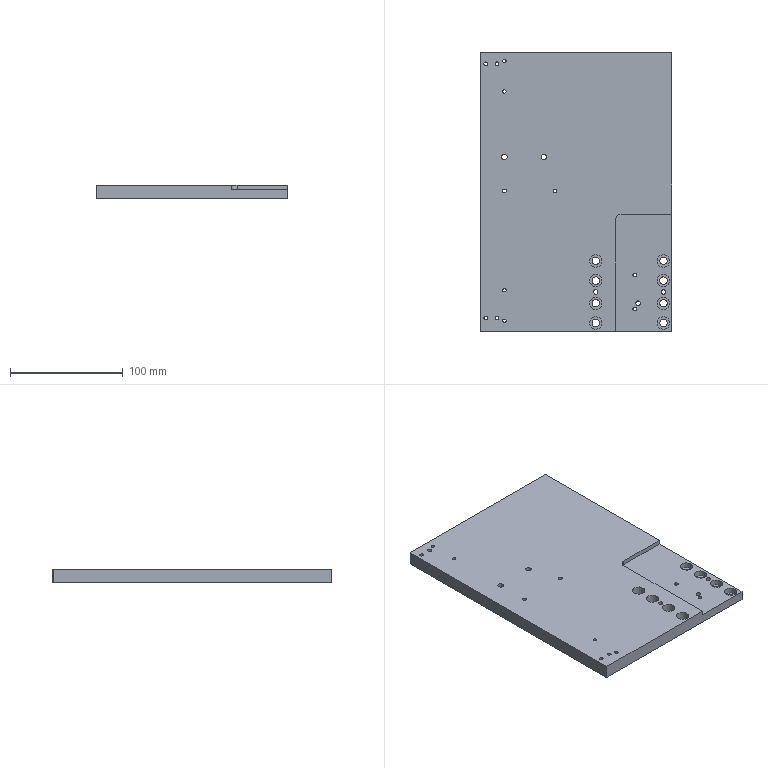Part | 1 solid | 53 faces | box 170 x 247.2 x 12 mm | volume 475967 mm3 | cylinder 34 | plane 19 | commonest cylinder face diameters 3.3 x8 6.6 x8 11 x8 3 x4 4 x3 5 x2
STEP:
#1=CARTESIAN_POINT('',(84.5,-91.3,8.1));
#2=VERTEX_POINT('',#1);
#3=CARTESIAN_POINT('',(85.,-90.8,8.1));
#4=VERTEX_POINT('',#3);
#5=CARTESIAN_POINT('',(85.,-90.8,8.1));
#6=DIRECTION('',(0.7071,0.7071,0.));
#7=VECTOR('',#6,1000.);
#8=LINE('',#5,#7);
#9=EDGE_CURVE('',#2,#4,#8,.T.);
#10=ORIENTED_EDGE('',*,*,#9,.F.);
#11=CARTESIAN_POINT('',(84.5,-91.3,0.));
#12=VERTEX_POINT('',#11);
#13=CARTESIAN_POINT('',(84.5,-91.3,12.));
#14=DIRECTION('',(0.,0.,1.));
#15=VECTOR('',#14,1000.);
#16=LINE('',#13,#15);
#17=EDGE_CURVE('',#12,#2,#16,.T.);
#18=ORIENTED_EDGE('',*,*,#17,.F.);
#19=CARTESIAN_POINT('',(85.,-90.8,0.));
#20=VERTEX_POINT('',#19);
#21=CARTESIAN_POINT('',(87.9,-87.9,0.));
#22=DIRECTION('',(-0.7071,-0.7071,0.));
#23=VECTOR('',#22,1000.);
#24=LINE('',#21,#23);
#25=EDGE_CURVE('',#20,#12,#24,.T.);
#26=ORIENTED_EDGE('',*,*,#25,.F.);
#27=CARTESIAN_POINT('',(85.,-90.8,12.));
#28=DIRECTION('',(0.,0.,-1.));
#29=VECTOR('',#28,1000.);
#30=LINE('',#27,#29);
#31=EDGE_CURVE('',#4,#20,#30,.T.);
#32=ORIENTED_EDGE('',*,*,#31,.F.);
#33=EDGE_LOOP('',(#10,#18,#26,#32));
#34=FACE_BOUND('',#33,.T.);
#35=CARTESIAN_POINT('',(85.,-90.8,12.));
#36=DIRECTION('',(-0.7071,0.7071,0.));
#37=DIRECTION('',(0.,0.,-1.));
#38=AXIS2_PLACEMENT_3D('',#35,#36,#37);
#39=PLANE('',#38);
#40=ADVANCED_FACE('',(#34),#39,.F.);
#41=CARTESIAN_POINT('',(-85.,155.4,0.));
#42=VERTEX_POINT('',#41);
#43=CARTESIAN_POINT('',(-84.5,155.9,0.));
#44=VERTEX_POINT('',#43);
#45=CARTESIAN_POINT('',(-120.2,120.2,0.));
#46=DIRECTION('',(0.7071,0.7071,0.));
#47=VECTOR('',#46,1000.);
#48=LINE('',#45,#47);
#49=EDGE_CURVE('',#42,#44,#48,.T.);
#50=ORIENTED_EDGE('',*,*,#49,.F.);
#51=CARTESIAN_POINT('',(-85.,155.4,12.));
#52=VERTEX_POINT('',#51);
#53=CARTESIAN_POINT('',(-85.,155.4,0.));
#54=DIRECTION('',(0.,0.,-1.));
#55=VECTOR('',#54,1000.);
#56=LINE('',#53,#55);
#57=EDGE_CURVE('',#52,#42,#56,.T.);
#58=ORIENTED_EDGE('',*,*,#57,.F.);
#59=CARTESIAN_POINT('',(-84.5,155.9,12.));
#60=VERTEX_POINT('',#59);
#61=CARTESIAN_POINT('',(-84.5,155.9,12.));
#62=DIRECTION('',(-0.7071,-0.7071,0.));
#63=VECTOR('',#62,1000.);
#64=LINE('',#61,#63);
#65=EDGE_CURVE('',#60,#52,#64,.T.);
#66=ORIENTED_EDGE('',*,*,#65,.F.);
#67=CARTESIAN_POINT('',(-84.5,155.9,12.));
#68=DIRECTION('',(0.,0.,1.));
#69=VECTOR('',#68,1000.);
#70=LINE('',#67,#69);
#71=EDGE_CURVE('',#44,#60,#70,.T.);
#72=ORIENTED_EDGE('',*,*,#71,.F.);
#73=EDGE_LOOP('',(#50,#58,#66,#72));
#74=FACE_BOUND('',#73,.T.);
#75=CARTESIAN_POINT('',(-84.5,155.9,-69.269));
#76=DIRECTION('',(-0.7071,0.7071,0.));
#77=DIRECTION('',(0.,0.,-1.));
#78=AXIS2_PLACEMENT_3D('',#75,#76,#77);
#79=PLANE('',#78);
#80=ADVANCED_FACE('',(#74),#79,.T.);
#81=CARTESIAN_POINT('',(85.,155.9,12.));
#82=VERTEX_POINT('',#81);
#83=CARTESIAN_POINT('',(-85.,155.9,12.));
#84=DIRECTION('',(-1.,0.,0.));
#85=VECTOR('',#84,1000.);
#86=LINE('',#83,#85);
#87=EDGE_CURVE('',#82,#60,#86,.T.);
#88=ORIENTED_EDGE('',*,*,#87,.F.);
#89=CARTESIAN_POINT('',(85.,155.9,0.));
#90=VERTEX_POINT('',#89);
#91=CARTESIAN_POINT('',(85.,155.9,-69.269));
#92=DIRECTION('',(0.,0.,1.));
#93=VECTOR('',#92,1000.);
#94=LINE('',#91,#93);
#95=EDGE_CURVE('',#90,#82,#94,.T.);
#96=ORIENTED_EDGE('',*,*,#95,.F.);
#97=CARTESIAN_POINT('',(-85.,155.9,0.));
#98=DIRECTION('',(-1.,0.,0.));
#99=VECTOR('',#98,1000.);
#100=LINE('',#97,#99);
#101=EDGE_CURVE('',#90,#44,#100,.T.);
#102=ORIENTED_EDGE('',*,*,#101,.T.);
#103=ORIENTED_EDGE('',*,*,#71,.T.);
#104=EDGE_LOOP('',(#88,#96,#102,#103));
#105=FACE_BOUND('',#104,.T.);
#106=CARTESIAN_POINT('',(-85.,155.9,-69.269));
#107=DIRECTION('',(0.,1.,0.));
#108=DIRECTION('',(0.,0.,1.));
#109=AXIS2_PLACEMENT_3D('',#106,#107,#108);
#110=PLANE('',#109);
#111=ADVANCED_FACE('',(#105),#110,.T.);
#112=CARTESIAN_POINT('',(35.1,7.7,8.1));
#113=VERTEX_POINT('',#112);
#114=CARTESIAN_POINT('',(35.1,-91.3,8.1));
#115=VERTEX_POINT('',#114);
#116=CARTESIAN_POINT('',(35.1,0.,8.1));
#117=DIRECTION('',(0.,-1.,0.));
#118=VECTOR('',#117,1000.);
#119=LINE('',#116,#118);
#120=EDGE_CURVE('',#113,#115,#119,.T.);
#121=ORIENTED_EDGE('',*,*,#120,.F.);
#122=CARTESIAN_POINT('',(35.1,7.7,12.));
#123=VERTEX_POINT('',#122);
#124=CARTESIAN_POINT('',(35.1,7.7,8.));
#125=DIRECTION('',(0.,0.,1.));
#126=VECTOR('',#125,1000.);
#127=LINE('',#124,#126);
#128=EDGE_CURVE('',#113,#123,#127,.T.);
#129=ORIENTED_EDGE('',*,*,#128,.T.);
#130=CARTESIAN_POINT('',(35.1,-91.3,12.));
#131=VERTEX_POINT('',#130);
#132=CARTESIAN_POINT('',(35.1,-91.3,12.));
#133=DIRECTION('',(0.,-1.,0.));
#134=VECTOR('',#133,1000.);
#135=LINE('',#132,#134);
#136=EDGE_CURVE('',#123,#131,#135,.T.);
#137=ORIENTED_EDGE('',*,*,#136,.T.);
#138=CARTESIAN_POINT('',(35.1,-91.3,12.));
#139=DIRECTION('',(0.,0.,1.));
#140=VECTOR('',#139,1000.);
#141=LINE('',#138,#140);
#142=EDGE_CURVE('',#115,#131,#141,.T.);
#143=ORIENTED_EDGE('',*,*,#142,.F.);
#144=EDGE_LOOP('',(#121,#129,#137,#143));
#145=FACE_BOUND('',#144,.T.);
#146=CARTESIAN_POINT('',(35.1,-91.3,8.));
#147=DIRECTION('',(-1.,0.,0.));
#148=DIRECTION('',(0.,0.,1.));
#149=AXIS2_PLACEMENT_3D('',#146,#147,#148);
#150=PLANE('',#149);
#151=ADVANCED_FACE('',(#145),#150,.F.);
#152=CARTESIAN_POINT('',(40.1,12.7,8.1));
#153=VERTEX_POINT('',#152);
#154=CARTESIAN_POINT('',(85.,12.7,8.1));
#155=VERTEX_POINT('',#154);
#156=CARTESIAN_POINT('',(0.,12.7,8.1));
#157=DIRECTION('',(1.,0.,0.));
#158=VECTOR('',#157,1000.);
#159=LINE('',#156,#158);
#160=EDGE_CURVE('',#153,#155,#159,.T.);
#161=ORIENTED_EDGE('',*,*,#160,.F.);
#162=CARTESIAN_POINT('',(40.1,7.7,8.1));
#163=DIRECTION('',(0.,0.,1.));
#164=DIRECTION('',(1.,0.,0.));
#165=AXIS2_PLACEMENT_3D('',#162,#163,#164);
#166=CIRCLE('',#165,5.);
#167=EDGE_CURVE('',#153,#113,#166,.T.);
#168=ORIENTED_EDGE('',*,*,#167,.T.);
#169=ORIENTED_EDGE('',*,*,#120,.T.);
#170=CARTESIAN_POINT('',(-85.,-91.3,8.1));
#171=DIRECTION('',(1.,0.,0.));
#172=VECTOR('',#171,1000.);
#173=LINE('',#170,#172);
#174=EDGE_CURVE('',#115,#2,#173,.T.);
#175=ORIENTED_EDGE('',*,*,#174,.T.);
#176=ORIENTED_EDGE('',*,*,#9,.T.);
#177=CARTESIAN_POINT('',(85.,-91.3,8.1));
#178=DIRECTION('',(0.,1.,0.));
#179=VECTOR('',#178,1000.);
#180=LINE('',#177,#179);
#181=EDGE_CURVE('',#4,#155,#180,.T.);
#182=ORIENTED_EDGE('',*,*,#181,.T.);
#183=EDGE_LOOP('',(#161,#168,#169,#175,#176,#182));
#184=FACE_BOUND('',#183,.T.);
#185=CARTESIAN_POINT('',(83.,-28.8,8.1));
#186=VERTEX_POINT('',#185);
#187=CARTESIAN_POINT('',(77.5,-28.8,8.1));
#188=DIRECTION('',(0.,0.,1.));
#189=DIRECTION('',(1.,0.,0.));
#190=AXIS2_PLACEMENT_3D('',#187,#188,#189);
#191=CIRCLE('',#190,5.5);
#192=EDGE_CURVE('',#186,#186,#191,.F.);
#193=ORIENTED_EDGE('',*,*,#192,.T.);
#194=EDGE_LOOP('',(#193));
#195=FACE_BOUND('',#194,.T.);
#196=CARTESIAN_POINT('',(83.,-83.8,8.1));
#197=VERTEX_POINT('',#196);
#198=CARTESIAN_POINT('',(77.5,-83.8,8.1));
#199=DIRECTION('',(0.,0.,1.));
#200=DIRECTION('',(1.,0.,0.));
#201=AXIS2_PLACEMENT_3D('',#198,#199,#200);
#202=CIRCLE('',#201,5.5);
#203=EDGE_CURVE('',#197,#197,#202,.F.);
#204=ORIENTED_EDGE('',*,*,#203,.T.);
#205=EDGE_LOOP('',(#204));
#206=FACE_BOUND('',#205,.T.);
#207=CARTESIAN_POINT('',(83.,-46.3,8.1));
#208=VERTEX_POINT('',#207);
#209=CARTESIAN_POINT('',(77.5,-46.3,8.1));
#210=DIRECTION('',(0.,0.,1.));
#211=DIRECTION('',(1.,0.,0.));
#212=AXIS2_PLACEMENT_3D('',#209,#210,#211);
#213=CIRCLE('',#212,5.5);
#214=EDGE_CURVE('',#208,#208,#213,.F.);
#215=ORIENTED_EDGE('',*,*,#214,.T.);
#216=EDGE_LOOP('',(#215));
#217=FACE_BOUND('',#216,.T.);
#218=CARTESIAN_POINT('',(83.,-66.3,8.1));
#219=VERTEX_POINT('',#218);
#220=CARTESIAN_POINT('',(77.5,-66.3,8.1));
#221=DIRECTION('',(0.,0.,1.));
#222=DIRECTION('',(1.,0.,0.));
#223=AXIS2_PLACEMENT_3D('',#220,#221,#222);
#224=CIRCLE('',#223,5.5);
#225=EDGE_CURVE('',#219,#219,#224,.F.);
#226=ORIENTED_EDGE('',*,*,#225,.T.);
#227=EDGE_LOOP('',(#226));
#228=FACE_BOUND('',#227,.T.);
#229=CARTESIAN_POINT('',(57.,-66.3,8.1));
#230=VERTEX_POINT('',#229);
#231=CARTESIAN_POINT('',(55.,-66.3,8.1));
#232=DIRECTION('',(0.,0.,1.));
#233=DIRECTION('',(1.,0.,0.));
#234=AXIS2_PLACEMENT_3D('',#231,#232,#233);
#235=CIRCLE('',#234,2.);
#236=EDGE_CURVE('',#230,#230,#235,.F.);
#237=ORIENTED_EDGE('',*,*,#236,.T.);
#238=EDGE_LOOP('',(#237));
#239=FACE_BOUND('',#238,.T.);
#240=CARTESIAN_POINT('',(79.5,-56.3,8.1));
#241=VERTEX_POINT('',#240);
#242=CARTESIAN_POINT('',(77.5,-56.3,8.1));
#243=DIRECTION('',(0.,0.,1.));
#244=DIRECTION('',(1.,0.,0.));
#245=AXIS2_PLACEMENT_3D('',#242,#243,#244);
#246=CIRCLE('',#245,2.);
#247=EDGE_CURVE('',#241,#241,#246,.F.);
#248=ORIENTED_EDGE('',*,*,#247,.T.);
#249=EDGE_LOOP('',(#248));
#250=FACE_BOUND('',#249,.T.);
#251=CARTESIAN_POINT('',(53.65,-41.3,8.1));
#252=VERTEX_POINT('',#251);
#253=CARTESIAN_POINT('',(52.,-41.3,8.1));
#254=DIRECTION('',(0.,0.,1.));
#255=DIRECTION('',(1.,0.,0.));
#256=AXIS2_PLACEMENT_3D('',#253,#254,#255);
#257=CIRCLE('',#256,1.65);
#258=EDGE_CURVE('',#252,#252,#257,.T.);
#259=ORIENTED_EDGE('',*,*,#258,.F.);
#260=EDGE_LOOP('',(#259));
#261=FACE_BOUND('',#260,.T.);
#262=CARTESIAN_POINT('',(53.65,-71.3,8.1));
#263=VERTEX_POINT('',#262);
#264=CARTESIAN_POINT('',(52.,-71.3,8.1));
#265=DIRECTION('',(0.,0.,1.));
#266=DIRECTION('',(1.,0.,0.));
#267=AXIS2_PLACEMENT_3D('',#264,#265,#266);
#268=CIRCLE('',#267,1.65);
#269=EDGE_CURVE('',#263,#263,#268,.T.);
#270=ORIENTED_EDGE('',*,*,#269,.F.);
#271=EDGE_LOOP('',(#270));
#272=FACE_BOUND('',#271,.T.);
#273=CARTESIAN_POINT('',(0.,0.,8.1));
#274=DIRECTION('',(0.,0.,1.));
#275=DIRECTION('',(1.,0.,0.));
#276=AXIS2_PLACEMENT_3D('',#273,#274,#275);
#277=PLANE('',#276);
#278=ADVANCED_FACE('',(#184,#195,#206,#217,#228,#239,#250,#261,#272),#277,.T.);
#279=CARTESIAN_POINT('',(83.,-66.3,3.));
#280=VERTEX_POINT('',#279);
#281=CARTESIAN_POINT('',(77.5,-66.3,3.));
#282=DIRECTION('',(0.,0.,1.));
#283=DIRECTION('',(1.,0.,0.));
#284=AXIS2_PLACEMENT_3D('',#281,#282,#283);
#285=CIRCLE('',#284,5.5);
#286=EDGE_CURVE('',#280,#280,#285,.T.);
#287=ORIENTED_EDGE('',*,*,#286,.T.);
#288=EDGE_LOOP('',(#287));
#289=FACE_BOUND('',#288,.T.);
#290=CARTESIAN_POINT('',(80.8,-66.3,3.));
#291=VERTEX_POINT('',#290);
#292=CARTESIAN_POINT('',(77.5,-66.3,3.));
#293=DIRECTION('',(0.,0.,1.));
#294=DIRECTION('',(1.,0.,0.));
#295=AXIS2_PLACEMENT_3D('',#292,#293,#294);
#296=CIRCLE('',#295,3.3);
#297=EDGE_CURVE('',#291,#291,#296,.T.);
#298=ORIENTED_EDGE('',*,*,#297,.F.);
#299=EDGE_LOOP('',(#298));
#300=FACE_BOUND('',#299,.T.);
#301=CARTESIAN_POINT('',(80.8,-66.3,3.));
#302=DIRECTION('',(0.,0.,-1.));
#303=DIRECTION('',(-1.,0.,0.));
#304=AXIS2_PLACEMENT_3D('',#301,#302,#303);
#305=PLANE('',#304);
#306=ADVANCED_FACE('',(#289,#300),#305,.F.);
#307=CARTESIAN_POINT('',(72.,-46.3,3.));
#308=VERTEX_POINT('',#307);
#309=CARTESIAN_POINT('',(77.5,-46.3,3.));
#310=DIRECTION('',(0.,0.,1.));
#311=DIRECTION('',(-1.,0.,0.));
#312=AXIS2_PLACEMENT_3D('',#309,#310,#311);
#313=CIRCLE('',#312,5.5);
#314=EDGE_CURVE('',#308,#308,#313,.T.);
#315=ORIENTED_EDGE('',*,*,#314,.T.);
#316=EDGE_LOOP('',(#315));
#317=FACE_BOUND('',#316,.T.);
#318=CARTESIAN_POINT('',(74.2,-46.3,3.));
#319=VERTEX_POINT('',#318);
#320=CARTESIAN_POINT('',(77.5,-46.3,3.));
#321=DIRECTION('',(0.,0.,1.));
#322=DIRECTION('',(-1.,0.,0.));
#323=AXIS2_PLACEMENT_3D('',#320,#321,#322);
#324=CIRCLE('',#323,3.3);
#325=EDGE_CURVE('',#319,#319,#324,.T.);
#326=ORIENTED_EDGE('',*,*,#325,.F.);
#327=EDGE_LOOP('',(#326));
#328=FACE_BOUND('',#327,.T.);
#329=CARTESIAN_POINT('',(80.8,-66.3,3.));
#330=DIRECTION('',(0.,0.,-1.));
#331=DIRECTION('',(-1.,0.,0.));
#332=AXIS2_PLACEMENT_3D('',#329,#330,#331);
#333=PLANE('',#332);
#334=ADVANCED_FACE('',(#317,#328),#333,.F.);
#335=CARTESIAN_POINT('',(12.,-66.3,3.));
#336=VERTEX_POINT('',#335);
#337=CARTESIAN_POINT('',(17.5,-66.3,3.));
#338=DIRECTION('',(0.,0.,1.));
#339=DIRECTION('',(-1.,0.,0.));
#340=AXIS2_PLACEMENT_3D('',#337,#338,#339);
#341=CIRCLE('',#340,5.5);
#342=EDGE_CURVE('',#336,#336,#341,.T.);
#343=ORIENTED_EDGE('',*,*,#342,.T.);
#344=EDGE_LOOP('',(#343));
#345=FACE_BOUND('',#344,.T.);
#346=CARTESIAN_POINT('',(14.2,-66.3,3.));
#347=VERTEX_POINT('',#346);
#348=CARTESIAN_POINT('',(17.5,-66.3,3.));
#349=DIRECTION('',(0.,0.,1.));
#350=DIRECTION('',(-1.,0.,0.));
#351=AXIS2_PLACEMENT_3D('',#348,#349,#350);
#352=CIRCLE('',#351,3.3);
#353=EDGE_CURVE('',#347,#347,#352,.T.);
#354=ORIENTED_EDGE('',*,*,#353,.F.);
#355=EDGE_LOOP('',(#354));
#356=FACE_BOUND('',#355,.T.);
#357=CARTESIAN_POINT('',(80.8,-66.3,3.));
#358=DIRECTION('',(0.,0.,-1.));
#359=DIRECTION('',(-1.,0.,0.));
#360=AXIS2_PLACEMENT_3D('',#357,#358,#359);
#361=PLANE('',#360);
#362=ADVANCED_FACE('',(#345,#356),#361,.F.);
#363=CARTESIAN_POINT('',(12.,-46.3,3.));
#364=VERTEX_POINT('',#363);
#365=CARTESIAN_POINT('',(17.5,-46.3,3.));
#366=DIRECTION('',(0.,0.,1.));
#367=DIRECTION('',(-1.,0.,0.));
#368=AXIS2_PLACEMENT_3D('',#365,#366,#367);
#369=CIRCLE('',#368,5.5);
#370=EDGE_CURVE('',#364,#364,#369,.T.);
#371=ORIENTED_EDGE('',*,*,#370,.T.);
#372=EDGE_LOOP('',(#371));
#373=FACE_BOUND('',#372,.T.);
#374=CARTESIAN_POINT('',(14.2,-46.3,3.));
#375=VERTEX_POINT('',#374);
#376=CARTESIAN_POINT('',(17.5,-46.3,3.));
#377=DIRECTION('',(0.,0.,1.));
#378=DIRECTION('',(-1.,0.,0.));
#379=AXIS2_PLACEMENT_3D('',#376,#377,#378);
#380=CIRCLE('',#379,3.3);
#381=EDGE_CURVE('',#375,#375,#380,.T.);
#382=ORIENTED_EDGE('',*,*,#381,.F.);
#383=EDGE_LOOP('',(#382));
#384=FACE_BOUND('',#383,.T.);
#385=CARTESIAN_POINT('',(80.8,-66.3,3.));
#386=DIRECTION('',(0.,0.,-1.));
#387=DIRECTION('',(-1.,0.,0.));
#388=AXIS2_PLACEMENT_3D('',#385,#386,#387);
#389=PLANE('',#388);
#390=ADVANCED_FACE('',(#373,#384),#389,.F.);
#391=CARTESIAN_POINT('',(72.,-83.8,3.));
#392=VERTEX_POINT('',#391);
#393=CARTESIAN_POINT('',(77.5,-83.8,3.));
#394=DIRECTION('',(0.,0.,1.));
#395=DIRECTION('',(-1.,0.,0.));
#396=AXIS2_PLACEMENT_3D('',#393,#394,#395);
#397=CIRCLE('',#396,5.5);
#398=EDGE_CURVE('',#392,#392,#397,.T.);
#399=ORIENTED_EDGE('',*,*,#398,.T.);
#400=EDGE_LOOP('',(#399));
#401=FACE_BOUND('',#400,.T.);
#402=CARTESIAN_POINT('',(74.2,-83.8,3.));
#403=VERTEX_POINT('',#402);
#404=CARTESIAN_POINT('',(77.5,-83.8,3.));
#405=DIRECTION('',(0.,0.,1.));
#406=DIRECTION('',(-1.,0.,0.));
#407=AXIS2_PLACEMENT_3D('',#404,#405,#406);
#408=CIRCLE('',#407,3.3);
#409=EDGE_CURVE('',#403,#403,#408,.T.);
#410=ORIENTED_EDGE('',*,*,#409,.F.);
#411=EDGE_LOOP('',(#410));
#412=FACE_BOUND('',#411,.T.);
#413=CARTESIAN_POINT('',(80.8,-66.3,3.));
#414=DIRECTION('',(0.,0.,-1.));
#415=DIRECTION('',(-1.,0.,0.));
#416=AXIS2_PLACEMENT_3D('',#413,#414,#415);
#417=PLANE('',#416);
#418=ADVANCED_FACE('',(#401,#412),#417,.F.);
#419=CARTESIAN_POINT('',(12.,-83.8,3.));
#420=VERTEX_POINT('',#419);
#421=CARTESIAN_POINT('',(17.5,-83.8,3.));
#422=DIRECTION('',(0.,0.,1.));
#423=DIRECTION('',(-1.,0.,0.));
#424=AXIS2_PLACEMENT_3D('',#421,#422,#423);
#425=CIRCLE('',#424,5.5);
#426=EDGE_CURVE('',#420,#420,#425,.T.);
#427=ORIENTED_EDGE('',*,*,#426,.T.);
#428=EDGE_LOOP('',(#427));
#429=FACE_BOUND('',#428,.T.);
#430=CARTESIAN_POINT('',(14.2,-83.8,3.));
#431=VERTEX_POINT('',#430);
#432=CARTESIAN_POINT('',(17.5,-83.8,3.));
#433=DIRECTION('',(0.,0.,1.));
#434=DIRECTION('',(-1.,0.,0.));
#435=AXIS2_PLACEMENT_3D('',#432,#433,#434);
#436=CIRCLE('',#435,3.3);
#437=EDGE_CURVE('',#431,#431,#436,.T.);
#438=ORIENTED_EDGE('',*,*,#437,.F.);
#439=EDGE_LOOP('',(#438));
#440=FACE_BOUND('',#439,.T.);
#441=CARTESIAN_POINT('',(80.8,-66.3,3.));
#442=DIRECTION('',(0.,0.,-1.));
#443=DIRECTION('',(-1.,0.,0.));
#444=AXIS2_PLACEMENT_3D('',#441,#442,#443);
#445=PLANE('',#444);
#446=ADVANCED_FACE('',(#429,#440),#445,.F.);
#447=CARTESIAN_POINT('',(72.,-28.8,3.));
#448=VERTEX_POINT('',#447);
#449=CARTESIAN_POINT('',(77.5,-28.8,3.));
#450=DIRECTION('',(0.,0.,1.));
#451=DIRECTION('',(-1.,0.,0.));
#452=AXIS2_PLACEMENT_3D('',#449,#450,#451);
#453=CIRCLE('',#452,5.5);
#454=EDGE_CURVE('',#448,#448,#453,.T.);
#455=ORIENTED_EDGE('',*,*,#454,.T.);
#456=EDGE_LOOP('',(#455));
#457=FACE_BOUND('',#456,.T.);
#458=CARTESIAN_POINT('',(74.2,-28.8,3.));
#459=VERTEX_POINT('',#458);
#460=CARTESIAN_POINT('',(77.5,-28.8,3.));
#461=DIRECTION('',(0.,0.,1.));
#462=DIRECTION('',(-1.,0.,0.));
#463=AXIS2_PLACEMENT_3D('',#460,#461,#462);
#464=CIRCLE('',#463,3.3);
#465=EDGE_CURVE('',#459,#459,#464,.T.);
#466=ORIENTED_EDGE('',*,*,#465,.F.);
#467=EDGE_LOOP('',(#466));
#468=FACE_BOUND('',#467,.T.);
#469=CARTESIAN_POINT('',(80.8,-66.3,3.));
#470=DIRECTION('',(0.,0.,-1.));
#471=DIRECTION('',(-1.,0.,0.));
#472=AXIS2_PLACEMENT_3D('',#469,#470,#471);
#473=PLANE('',#472);
#474=ADVANCED_FACE('',(#457,#468),#473,.F.);
#475=CARTESIAN_POINT('',(12.,-28.8,3.));
#476=VERTEX_POINT('',#475);
#477=CARTESIAN_POINT('',(17.5,-28.8,3.));
#478=DIRECTION('',(0.,0.,1.));
#479=DIRECTION('',(-1.,0.,0.));
#480=AXIS2_PLACEMENT_3D('',#477,#478,#479);
#481=CIRCLE('',#480,5.5);
#482=EDGE_CURVE('',#476,#476,#481,.T.);
#483=ORIENTED_EDGE('',*,*,#482,.T.);
#484=EDGE_LOOP('',(#483));
#485=FACE_BOUND('',#484,.T.);
#486=CARTESIAN_POINT('',(14.2,-28.8,3.));
#487=VERTEX_POINT('',#486);
#488=CARTESIAN_POINT('',(17.5,-28.8,3.));
#489=DIRECTION('',(0.,0.,1.));
#490=DIRECTION('',(-1.,0.,0.));
#491=AXIS2_PLACEMENT_3D('',#488,#489,#490);
#492=CIRCLE('',#491,3.3);
#493=EDGE_CURVE('',#487,#487,#492,.T.);
#494=ORIENTED_EDGE('',*,*,#493,.F.);
#495=EDGE_LOOP('',(#494));
#496=FACE_BOUND('',#495,.T.);
#497=CARTESIAN_POINT('',(80.8,-66.3,3.));
#498=DIRECTION('',(0.,0.,-1.));
#499=DIRECTION('',(-1.,0.,0.));
#500=AXIS2_PLACEMENT_3D('',#497,#498,#499);
#501=PLANE('',#500);
#502=ADVANCED_FACE('',(#485,#496),#501,.F.);
#503=CARTESIAN_POINT('',(-85.,-91.3,0.));
#504=VERTEX_POINT('',#503);
#505=CARTESIAN_POINT('',(-85.,-91.3,0.));
#506=DIRECTION('',(1.,0.,0.));
#507=VECTOR('',#506,1000.);
#508=LINE('',#505,#507);
#509=EDGE_CURVE('',#504,#12,#508,.T.);
#510=ORIENTED_EDGE('',*,*,#509,.T.);
#511=ORIENTED_EDGE('',*,*,#17,.T.);
#512=ORIENTED_EDGE('',*,*,#174,.F.);
#513=ORIENTED_EDGE('',*,*,#142,.T.);
#514=CARTESIAN_POINT('',(-85.,-91.3,12.));
#515=VERTEX_POINT('',#514);
#516=CARTESIAN_POINT('',(-85.,-91.3,12.));
#517=DIRECTION('',(1.,0.,0.));
#518=VECTOR('',#517,1000.);
#519=LINE('',#516,#518);
#520=EDGE_CURVE('',#515,#131,#519,.T.);
#521=ORIENTED_EDGE('',*,*,#520,.F.);
#522=CARTESIAN_POINT('',(-85.,-91.3,12.));
#523=DIRECTION('',(0.,0.,-1.));
#524=VECTOR('',#523,1000.);
#525=LINE('',#522,#524);
#526=EDGE_CURVE('',#515,#504,#525,.T.);
#527=ORIENTED_EDGE('',*,*,#526,.T.);
#528=EDGE_LOOP('',(#510,#511,#512,#513,#521,#527));
#529=FACE_BOUND('',#528,.T.);
#530=CARTESIAN_POINT('',(-85.,-91.3,12.));
#531=DIRECTION('',(0.,1.,0.));
#532=DIRECTION('',(0.,0.,1.));
#533=AXIS2_PLACEMENT_3D('',#530,#531,#532);
#534=PLANE('',#533);
#535=ADVANCED_FACE('',(#529),#534,.F.);
#536=CARTESIAN_POINT('',(-85.,-91.3,12.));
#537=DIRECTION('',(0.,-1.,0.));
#538=VECTOR('',#537,1000.);
#539=LINE('',#536,#538);
#540=EDGE_CURVE('',#52,#515,#539,.T.);
#541=ORIENTED_EDGE('',*,*,#540,.F.);
#542=ORIENTED_EDGE('',*,*,#57,.T.);
#543=CARTESIAN_POINT('',(-85.,-91.3,0.));
#544=DIRECTION('',(0.,-1.,0.));
#545=VECTOR('',#544,1000.);
#546=LINE('',#543,#545);
#547=EDGE_CURVE('',#42,#504,#546,.T.);
#548=ORIENTED_EDGE('',*,*,#547,.T.);
#549=ORIENTED_EDGE('',*,*,#526,.F.);
#550=EDGE_LOOP('',(#541,#542,#548,#549));
#551=FACE_BOUND('',#550,.T.);
#552=CARTESIAN_POINT('',(-85.,-91.3,12.));
#553=DIRECTION('',(1.,0.,0.));
#554=DIRECTION('',(0.,0.,-1.));
#555=AXIS2_PLACEMENT_3D('',#552,#553,#554);
#556=PLANE('',#555);
#557=ADVANCED_FACE('',(#551),#556,.F.);
#558=CARTESIAN_POINT('',(85.,-91.3,0.));
#559=DIRECTION('',(0.,1.,0.));
#560=VECTOR('',#559,1000.);
#561=LINE('',#558,#560);
#562=EDGE_CURVE('',#20,#90,#561,.T.);
#563=ORIENTED_EDGE('',*,*,#562,.T.);
#564=ORIENTED_EDGE('',*,*,#95,.T.);
#565=CARTESIAN_POINT('',(85.,12.7,12.));
#566=VERTEX_POINT('',#565);
#567=CARTESIAN_POINT('',(85.,32.3,12.));
#568=DIRECTION('',(0.,-1.,0.));
#569=VECTOR('',#568,1000.);
#570=LINE('',#567,#569);
#571=EDGE_CURVE('',#82,#566,#570,.T.);
#572=ORIENTED_EDGE('',*,*,#571,.T.);
#573=CARTESIAN_POINT('',(85.,12.7,8.));
#574=DIRECTION('',(0.,0.,1.));
#575=VECTOR('',#574,1000.);
#576=LINE('',#573,#575);
#577=EDGE_CURVE('',#155,#566,#576,.T.);
#578=ORIENTED_EDGE('',*,*,#577,.F.);
#579=ORIENTED_EDGE('',*,*,#181,.F.);
#580=ORIENTED_EDGE('',*,*,#31,.T.);
#581=EDGE_LOOP('',(#563,#564,#572,#578,#579,#580));
#582=FACE_BOUND('',#581,.T.);
#583=CARTESIAN_POINT('',(85.,-91.3,12.));
#584=DIRECTION('',(-1.,0.,0.));
#585=DIRECTION('',(0.,0.,1.));
#586=AXIS2_PLACEMENT_3D('',#583,#584,#585);
#587=PLANE('',#586);
#588=ADVANCED_FACE('',(#582),#587,.F.);
#589=ORIENTED_EDGE('',*,*,#136,.F.);
#590=CARTESIAN_POINT('',(40.1,12.7,12.));
#591=VERTEX_POINT('',#590);
#592=CARTESIAN_POINT('',(40.1,7.7,12.));
#593=DIRECTION('',(0.,0.,-1.));
#594=DIRECTION('',(-1.,0.,0.));
#595=AXIS2_PLACEMENT_3D('',#592,#593,#594);
#596=CIRCLE('',#595,5.);
#597=EDGE_CURVE('',#123,#591,#596,.T.);
#598=ORIENTED_EDGE('',*,*,#597,.T.);
#599=CARTESIAN_POINT('',(60.,12.7,12.));
#600=DIRECTION('',(-1.,0.,0.));
#601=VECTOR('',#600,1000.);
#602=LINE('',#599,#601);
#603=EDGE_CURVE('',#566,#591,#602,.T.);
#604=ORIENTED_EDGE('',*,*,#603,.F.);
#605=ORIENTED_EDGE('',*,*,#571,.F.);
#606=ORIENTED_EDGE('',*,*,#87,.T.);
#607=ORIENTED_EDGE('',*,*,#65,.T.);
#608=ORIENTED_EDGE('',*,*,#540,.T.);
#609=ORIENTED_EDGE('',*,*,#520,.T.);
#610=EDGE_LOOP('',(#589,#598,#604,#605,#606,#607,#608,#609));
#611=FACE_BOUND('',#610,.T.);
#612=CARTESIAN_POINT('',(-68.35,145.9,12.));
#613=VERTEX_POINT('',#612);
#614=CARTESIAN_POINT('',(-70.,145.9,12.));
#615=DIRECTION('',(0.,0.,1.));
#616=DIRECTION('',(1.,0.,0.));
#617=AXIS2_PLACEMENT_3D('',#614,#615,#616);
#618=CIRCLE('',#617,1.65);
#619=EDGE_CURVE('',#613,#613,#618,.T.);
#620=ORIENTED_EDGE('',*,*,#619,.F.);
#621=EDGE_LOOP('',(#620));
#622=FACE_BOUND('',#621,.T.);
#623=CARTESIAN_POINT('',(-61.,63.3,12.));
#624=VERTEX_POINT('',#623);
#625=CARTESIAN_POINT('',(-63.5,63.3,12.));
#626=DIRECTION('',(0.,0.,1.));
#627=DIRECTION('',(1.,0.,0.));
#628=AXIS2_PLACEMENT_3D('',#625,#626,#627);
#629=CIRCLE('',#628,2.5);
#630=EDGE_CURVE('',#624,#624,#629,.T.);
#631=ORIENTED_EDGE('',*,*,#630,.F.);
#632=EDGE_LOOP('',(#631));
#633=FACE_BOUND('',#632,.T.);
#634=CARTESIAN_POINT('',(23.,-28.8,12.));
#635=VERTEX_POINT('',#634);
#636=CARTESIAN_POINT('',(17.5,-28.8,12.));
#637=DIRECTION('',(0.,0.,1.));
#638=DIRECTION('',(1.,0.,0.));
#639=AXIS2_PLACEMENT_3D('',#636,#637,#638);
#640=CIRCLE('',#639,5.5);
#641=EDGE_CURVE('',#635,#635,#640,.T.);
#642=ORIENTED_EDGE('',*,*,#641,.F.);
#643=EDGE_LOOP('',(#642));
#644=FACE_BOUND('',#643,.T.);
#645=CARTESIAN_POINT('',(23.,-83.8,12.));
#646=VERTEX_POINT('',#645);
#647=CARTESIAN_POINT('',(17.5,-83.8,12.));
#648=DIRECTION('',(0.,0.,1.));
#649=DIRECTION('',(1.,0.,0.));
#650=AXIS2_PLACEMENT_3D('',#647,#648,#649);
#651=CIRCLE('',#650,5.5);
#652=EDGE_CURVE('',#646,#646,#651,.T.);
#653=ORIENTED_EDGE('',*,*,#652,.F.);
#654=EDGE_LOOP('',(#653));
#655=FACE_BOUND('',#654,.T.);
#656=CARTESIAN_POINT('',(23.,-46.3,12.));
#657=VERTEX_POINT('',#656);
#658=CARTESIAN_POINT('',(17.5,-46.3,12.));
#659=DIRECTION('',(0.,0.,1.));
#660=DIRECTION('',(1.,0.,0.));
#661=AXIS2_PLACEMENT_3D('',#658,#659,#660);
#662=CIRCLE('',#661,5.5);
#663=EDGE_CURVE('',#657,#657,#662,.T.);
#664=ORIENTED_EDGE('',*,*,#663,.F.);
#665=EDGE_LOOP('',(#664));
#666=FACE_BOUND('',#665,.T.);
#667=CARTESIAN_POINT('',(23.,-66.3,12.));
#668=VERTEX_POINT('',#667);
#669=CARTESIAN_POINT('',(17.5,-66.3,12.));
#670=DIRECTION('',(0.,0.,1.));
#671=DIRECTION('',(1.,0.,0.));
#672=AXIS2_PLACEMENT_3D('',#669,#670,#671);
#673=CIRCLE('',#672,5.5);
#674=EDGE_CURVE('',#668,#668,#673,.T.);
#675=ORIENTED_EDGE('',*,*,#674,.F.);
#676=EDGE_LOOP('',(#675));
#677=FACE_BOUND('',#676,.T.);
#678=CARTESIAN_POINT('',(19.5,-56.3,12.));
#679=VERTEX_POINT('',#678);
#680=CARTESIAN_POINT('',(17.5,-56.3,12.));
#681=DIRECTION('',(0.,0.,1.));
#682=DIRECTION('',(1.,0.,0.));
#683=AXIS2_PLACEMENT_3D('',#680,#681,#682);
#684=CIRCLE('',#683,2.);
#685=EDGE_CURVE('',#679,#679,#684,.T.);
#686=ORIENTED_EDGE('',*,*,#685,.F.);
#687=EDGE_LOOP('',(#686));
#688=FACE_BOUND('',#687,.T.);
#689=CARTESIAN_POINT('',(-16.85,33.3,12.));
#690=VERTEX_POINT('',#689);
#691=CARTESIAN_POINT('',(-18.5,33.3,12.));
#692=DIRECTION('',(0.,0.,1.));
#693=DIRECTION('',(1.,0.,0.));
#694=AXIS2_PLACEMENT_3D('',#691,#692,#693);
#695=CIRCLE('',#694,1.65);
#696=EDGE_CURVE('',#690,#690,#695,.T.);
#697=ORIENTED_EDGE('',*,*,#696,.F.);
#698=EDGE_LOOP('',(#697));
#699=FACE_BOUND('',#698,.T.);
#700=CARTESIAN_POINT('',(-61.85,33.3,12.));
#701=VERTEX_POINT('',#700);
#702=CARTESIAN_POINT('',(-63.5,33.3,12.));
#703=DIRECTION('',(0.,0.,1.));
#704=DIRECTION('',(1.,0.,0.));
#705=AXIS2_PLACEMENT_3D('',#702,#703,#704);
#706=CIRCLE('',#705,1.65);
#707=EDGE_CURVE('',#701,#701,#706,.T.);
#708=ORIENTED_EDGE('',*,*,#707,.F.);
#709=EDGE_LOOP('',(#708));
#710=FACE_BOUND('',#709,.T.);
#711=CARTESIAN_POINT('',(-26.,63.3,12.));
#712=VERTEX_POINT('',#711);
#713=CARTESIAN_POINT('',(-28.5,63.3,12.));
#714=DIRECTION('',(0.,0.,1.));
#715=DIRECTION('',(1.,0.,0.));
#716=AXIS2_PLACEMENT_3D('',#713,#714,#715);
#717=CIRCLE('',#716,2.5);
#718=EDGE_CURVE('',#712,#712,#717,.T.);
#719=ORIENTED_EDGE('',*,*,#718,.F.);
#720=EDGE_LOOP('',(#719));
#721=FACE_BOUND('',#720,.T.);
#722=CARTESIAN_POINT('',(-78.35,145.9,12.));
#723=VERTEX_POINT('',#722);
#724=CARTESIAN_POINT('',(-80.,145.9,12.));
#725=DIRECTION('',(0.,0.,1.));
#726=DIRECTION('',(1.,0.,0.));
#727=AXIS2_PLACEMENT_3D('',#724,#725,#726);
#728=CIRCLE('',#727,1.65);
#729=EDGE_CURVE('',#723,#723,#728,.T.);
#730=ORIENTED_EDGE('',*,*,#729,.F.);
#731=EDGE_LOOP('',(#730));
#732=FACE_BOUND('',#731,.T.);
#733=CARTESIAN_POINT('',(-68.35,-79.3,12.));
#734=VERTEX_POINT('',#733);
#735=CARTESIAN_POINT('',(-70.,-79.3,12.));
#736=DIRECTION('',(0.,0.,1.));
#737=DIRECTION('',(1.,0.,0.));
#738=AXIS2_PLACEMENT_3D('',#735,#736,#737);
#739=CIRCLE('',#738,1.65);
#740=EDGE_CURVE('',#734,#734,#739,.T.);
#741=ORIENTED_EDGE('',*,*,#740,.F.);
#742=EDGE_LOOP('',(#741));
#743=FACE_BOUND('',#742,.T.);
#744=CARTESIAN_POINT('',(-78.35,-79.3,12.));
#745=VERTEX_POINT('',#744);
#746=CARTESIAN_POINT('',(-80.,-79.3,12.));
#747=DIRECTION('',(0.,0.,1.));
#748=DIRECTION('',(1.,0.,0.));
#749=AXIS2_PLACEMENT_3D('',#746,#747,#748);
#750=CIRCLE('',#749,1.65);
#751=EDGE_CURVE('',#745,#745,#750,.T.);
#752=ORIENTED_EDGE('',*,*,#751,.F.);
#753=EDGE_LOOP('',(#752));
#754=FACE_BOUND('',#753,.T.);
#755=CARTESIAN_POINT('',(-62.,121.4,12.));
#756=VERTEX_POINT('',#755);
#757=CARTESIAN_POINT('',(-63.5,121.4,12.));
#758=DIRECTION('',(0.,0.,1.));
#759=DIRECTION('',(1.,0.,0.));
#760=AXIS2_PLACEMENT_3D('',#757,#758,#759);
#761=CIRCLE('',#760,1.5);
#762=EDGE_CURVE('',#756,#756,#761,.T.);
#763=ORIENTED_EDGE('',*,*,#762,.F.);
#764=EDGE_LOOP('',(#763));
#765=FACE_BOUND('',#764,.T.);
#766=CARTESIAN_POINT('',(-62.,148.4,12.));
#767=VERTEX_POINT('',#766);
#768=CARTESIAN_POINT('',(-63.5,148.4,12.));
#769=DIRECTION('',(0.,0.,1.));
#770=DIRECTION('',(1.,0.,0.));
#771=AXIS2_PLACEMENT_3D('',#768,#769,#770);
#772=CIRCLE('',#771,1.5);
#773=EDGE_CURVE('',#767,#767,#772,.T.);
#774=ORIENTED_EDGE('',*,*,#773,.F.);
#775=EDGE_LOOP('',(#774));
#776=FACE_BOUND('',#775,.T.);
#777=CARTESIAN_POINT('',(-62.,-54.8,12.));
#778=VERTEX_POINT('',#777);
#779=CARTESIAN_POINT('',(-63.5,-54.8,12.));
#780=DIRECTION('',(0.,0.,1.));
#781=DIRECTION('',(1.,0.,0.));
#782=AXIS2_PLACEMENT_3D('',#779,#780,#781);
#783=CIRCLE('',#782,1.5);
#784=EDGE_CURVE('',#778,#778,#783,.T.);
#785=ORIENTED_EDGE('',*,*,#784,.F.);
#786=EDGE_LOOP('',(#785));
#787=FACE_BOUND('',#786,.T.);
#788=CARTESIAN_POINT('',(-62.,-81.8,12.));
#789=VERTEX_POINT('',#788);
#790=CARTESIAN_POINT('',(-63.5,-81.8,12.));
#791=DIRECTION('',(0.,0.,1.));
#792=DIRECTION('',(1.,0.,0.));
#793=AXIS2_PLACEMENT_3D('',#790,#791,#792);
#794=CIRCLE('',#793,1.5);
#795=EDGE_CURVE('',#789,#789,#794,.T.);
#796=ORIENTED_EDGE('',*,*,#795,.F.);
#797=EDGE_LOOP('',(#796));
#798=FACE_BOUND('',#797,.T.);
#799=CARTESIAN_POINT('',(0.,0.,12.));
#800=DIRECTION('',(0.,0.,-1.));
#801=DIRECTION('',(-1.,0.,0.));
#802=AXIS2_PLACEMENT_3D('',#799,#800,#801);
#803=PLANE('',#802);
#804=ADVANCED_FACE('',(#611,#622,#633,#644,#655,#666,#677,#688,#699,#710,#721,#732,#743,#754,#765,#776,#787,#798),#803,.F.);
#805=CARTESIAN_POINT('',(-78.35,-79.3,0.));
#806=VERTEX_POINT('',#805);
#807=CARTESIAN_POINT('',(-80.,-79.3,0.));
#808=DIRECTION('',(0.,0.,1.));
#809=DIRECTION('',(1.,0.,0.));
#810=AXIS2_PLACEMENT_3D('',#807,#808,#809);
#811=CIRCLE('',#810,1.65);
#812=EDGE_CURVE('',#806,#806,#811,.T.);
#813=ORIENTED_EDGE('',*,*,#812,.T.);
#814=EDGE_LOOP('',(#813));
#815=FACE_BOUND('',#814,.T.);
#816=CARTESIAN_POINT('',(-68.35,-79.3,0.));
#817=VERTEX_POINT('',#816);
#818=CARTESIAN_POINT('',(-70.,-79.3,0.));
#819=DIRECTION('',(0.,0.,1.));
#820=DIRECTION('',(1.,0.,0.));
#821=AXIS2_PLACEMENT_3D('',#818,#819,#820);
#822=CIRCLE('',#821,1.65);
#823=EDGE_CURVE('',#817,#817,#822,.T.);
#824=ORIENTED_EDGE('',*,*,#823,.T.);
#825=EDGE_LOOP('',(#824));
#826=FACE_BOUND('',#825,.T.);
#827=CARTESIAN_POINT('',(-68.35,145.9,0.));
#828=VERTEX_POINT('',#827);
#829=CARTESIAN_POINT('',(-70.,145.9,0.));
#830=DIRECTION('',(0.,0.,1.));
#831=DIRECTION('',(1.,0.,0.));
#832=AXIS2_PLACEMENT_3D('',#829,#830,#831);
#833=CIRCLE('',#832,1.65);
#834=EDGE_CURVE('',#828,#828,#833,.T.);
#835=ORIENTED_EDGE('',*,*,#834,.T.);
#836=EDGE_LOOP('',(#835));
#837=FACE_BOUND('',#836,.T.);
#838=CARTESIAN_POINT('',(80.8,-46.3,0.));
#839=VERTEX_POINT('',#838);
#840=CARTESIAN_POINT('',(77.5,-46.3,0.));
#841=DIRECTION('',(0.,0.,1.));
#842=DIRECTION('',(1.,0.,0.));
#843=AXIS2_PLACEMENT_3D('',#840,#841,#842);
#844=CIRCLE('',#843,3.3);
#845=EDGE_CURVE('',#839,#839,#844,.T.);
#846=ORIENTED_EDGE('',*,*,#845,.T.);
#847=EDGE_LOOP('',(#846));
#848=FACE_BOUND('',#847,.T.);
#849=CARTESIAN_POINT('',(20.8,-66.3,0.));
#850=VERTEX_POINT('',#849);
#851=CARTESIAN_POINT('',(17.5,-66.3,0.));
#852=DIRECTION('',(0.,0.,1.));
#853=DIRECTION('',(1.,0.,0.));
#854=AXIS2_PLACEMENT_3D('',#851,#852,#853);
#855=CIRCLE('',#854,3.3);
#856=EDGE_CURVE('',#850,#850,#855,.T.);
#857=ORIENTED_EDGE('',*,*,#856,.T.);
#858=EDGE_LOOP('',(#857));
#859=FACE_BOUND('',#858,.T.);
#860=CARTESIAN_POINT('',(20.8,-46.3,0.));
#861=VERTEX_POINT('',#860);
#862=CARTESIAN_POINT('',(17.5,-46.3,0.));
#863=DIRECTION('',(0.,0.,1.));
#864=DIRECTION('',(1.,0.,0.));
#865=AXIS2_PLACEMENT_3D('',#862,#863,#864);
#866=CIRCLE('',#865,3.3);
#867=EDGE_CURVE('',#861,#861,#866,.T.);
#868=ORIENTED_EDGE('',*,*,#867,.T.);
#869=EDGE_LOOP('',(#868));
#870=FACE_BOUND('',#869,.T.);
#871=CARTESIAN_POINT('',(80.8,-83.8,0.));
#872=VERTEX_POINT('',#871);
#873=CARTESIAN_POINT('',(77.5,-83.8,0.));
#874=DIRECTION('',(0.,0.,1.));
#875=DIRECTION('',(1.,0.,0.));
#876=AXIS2_PLACEMENT_3D('',#873,#874,#875);
#877=CIRCLE('',#876,3.3);
#878=EDGE_CURVE('',#872,#872,#877,.T.);
#879=ORIENTED_EDGE('',*,*,#878,.T.);
#880=EDGE_LOOP('',(#879));
#881=FACE_BOUND('',#880,.T.);
#882=CARTESIAN_POINT('',(20.8,-83.8,0.));
#883=VERTEX_POINT('',#882);
#884=CARTESIAN_POINT('',(17.5,-83.8,0.));
#885=DIRECTION('',(0.,0.,1.));
#886=DIRECTION('',(1.,0.,0.));
#887=AXIS2_PLACEMENT_3D('',#884,#885,#886);
#888=CIRCLE('',#887,3.3);
#889=EDGE_CURVE('',#883,#883,#888,.T.);
#890=ORIENTED_EDGE('',*,*,#889,.T.);
#891=EDGE_LOOP('',(#890));
#892=FACE_BOUND('',#891,.T.);
#893=CARTESIAN_POINT('',(80.8,-28.8,0.));
#894=VERTEX_POINT('',#893);
#895=CARTESIAN_POINT('',(77.5,-28.8,0.));
#896=DIRECTION('',(0.,0.,1.));
#897=DIRECTION('',(1.,0.,0.));
#898=AXIS2_PLACEMENT_3D('',#895,#896,#897);
#899=CIRCLE('',#898,3.3);
#900=EDGE_CURVE('',#894,#894,#899,.T.);
#901=ORIENTED_EDGE('',*,*,#900,.T.);
#902=EDGE_LOOP('',(#901));
#903=FACE_BOUND('',#902,.T.);
#904=CARTESIAN_POINT('',(20.8,-28.8,0.));
#905=VERTEX_POINT('',#904);
#906=CARTESIAN_POINT('',(17.5,-28.8,0.));
#907=DIRECTION('',(0.,0.,1.));
#908=DIRECTION('',(1.,0.,0.));
#909=AXIS2_PLACEMENT_3D('',#906,#907,#908);
#910=CIRCLE('',#909,3.3);
#911=EDGE_CURVE('',#905,#905,#910,.T.);
#912=ORIENTED_EDGE('',*,*,#911,.T.);
#913=EDGE_LOOP('',(#912));
#914=FACE_BOUND('',#913,.T.);
#915=CARTESIAN_POINT('',(80.8,-66.3,0.));
#916=VERTEX_POINT('',#915);
#917=CARTESIAN_POINT('',(77.5,-66.3,0.));
#918=DIRECTION('',(0.,0.,1.));
#919=DIRECTION('',(1.,0.,0.));
#920=AXIS2_PLACEMENT_3D('',#917,#918,#919);
#921=CIRCLE('',#920,3.3);
#922=EDGE_CURVE('',#916,#916,#921,.T.);
#923=ORIENTED_EDGE('',*,*,#922,.T.);
#924=EDGE_LOOP('',(#923));
#925=FACE_BOUND('',#924,.T.);
#926=CARTESIAN_POINT('',(57.,-66.3,0.));
#927=VERTEX_POINT('',#926);
#928=CARTESIAN_POINT('',(55.,-66.3,0.));
#929=DIRECTION('',(0.,0.,1.));
#930=DIRECTION('',(1.,0.,0.));
#931=AXIS2_PLACEMENT_3D('',#928,#929,#930);
#932=CIRCLE('',#931,2.);
#933=EDGE_CURVE('',#927,#927,#932,.T.);
#934=ORIENTED_EDGE('',*,*,#933,.T.);
#935=EDGE_LOOP('',(#934));
#936=FACE_BOUND('',#935,.T.);
#937=CARTESIAN_POINT('',(79.5,-56.3,0.));
#938=VERTEX_POINT('',#937);
#939=CARTESIAN_POINT('',(77.5,-56.3,0.));
#940=DIRECTION('',(0.,0.,1.));
#941=DIRECTION('',(1.,0.,0.));
#942=AXIS2_PLACEMENT_3D('',#939,#940,#941);
#943=CIRCLE('',#942,2.);
#944=EDGE_CURVE('',#938,#938,#943,.T.);
#945=ORIENTED_EDGE('',*,*,#944,.T.);
#946=EDGE_LOOP('',(#945));
#947=FACE_BOUND('',#946,.T.);
#948=CARTESIAN_POINT('',(19.5,-56.3,0.));
#949=VERTEX_POINT('',#948);
#950=CARTESIAN_POINT('',(17.5,-56.3,0.));
#951=DIRECTION('',(0.,0.,1.));
#952=DIRECTION('',(1.,0.,0.));
#953=AXIS2_PLACEMENT_3D('',#950,#951,#952);
#954=CIRCLE('',#953,2.);
#955=EDGE_CURVE('',#949,#949,#954,.T.);
#956=ORIENTED_EDGE('',*,*,#955,.T.);
#957=EDGE_LOOP('',(#956));
#958=FACE_BOUND('',#957,.T.);
#959=CARTESIAN_POINT('',(-16.85,33.3,0.));
#960=VERTEX_POINT('',#959);
#961=CARTESIAN_POINT('',(-18.5,33.3,0.));
#962=DIRECTION('',(0.,0.,1.));
#963=DIRECTION('',(1.,0.,0.));
#964=AXIS2_PLACEMENT_3D('',#961,#962,#963);
#965=CIRCLE('',#964,1.65);
#966=EDGE_CURVE('',#960,#960,#965,.T.);
#967=ORIENTED_EDGE('',*,*,#966,.T.);
#968=EDGE_LOOP('',(#967));
#969=FACE_BOUND('',#968,.T.);
#970=CARTESIAN_POINT('',(-61.85,33.3,0.));
#971=VERTEX_POINT('',#970);
#972=CARTESIAN_POINT('',(-63.5,33.3,0.));
#973=DIRECTION('',(0.,0.,1.));
#974=DIRECTION('',(1.,0.,0.));
#975=AXIS2_PLACEMENT_3D('',#972,#973,#974);
#976=CIRCLE('',#975,1.65);
#977=EDGE_CURVE('',#971,#971,#976,.T.);
#978=ORIENTED_EDGE('',*,*,#977,.T.);
#979=EDGE_LOOP('',(#978));
#980=FACE_BOUND('',#979,.T.);
#981=CARTESIAN_POINT('',(-26.,63.3,0.));
#982=VERTEX_POINT('',#981);
#983=CARTESIAN_POINT('',(-28.5,63.3,0.));
#984=DIRECTION('',(0.,0.,1.));
#985=DIRECTION('',(1.,0.,0.));
#986=AXIS2_PLACEMENT_3D('',#983,#984,#985);
#987=CIRCLE('',#986,2.5);
#988=EDGE_CURVE('',#982,#982,#987,.T.);
#989=ORIENTED_EDGE('',*,*,#988,.T.);
#990=EDGE_LOOP('',(#989));
#991=FACE_BOUND('',#990,.T.);
#992=CARTESIAN_POINT('',(-61.,63.3,0.));
#993=VERTEX_POINT('',#992);
#994=CARTESIAN_POINT('',(-63.5,63.3,0.));
#995=DIRECTION('',(0.,0.,1.));
#996=DIRECTION('',(1.,0.,0.));
#997=AXIS2_PLACEMENT_3D('',#994,#995,#996);
#998=CIRCLE('',#997,2.5);
#999=EDGE_CURVE('',#993,#993,#998,.T.);
#1000=ORIENTED_EDGE('',*,*,#999,.T.);
#1001=EDGE_LOOP('',(#1000));
#1002=FACE_BOUND('',#1001,.T.);
#1003=CARTESIAN_POINT('',(53.65,-41.3,0.));
#1004=VERTEX_POINT('',#1003);
#1005=CARTESIAN_POINT('',(52.,-41.3,0.));
#1006=DIRECTION('',(0.,0.,1.));
#1007=DIRECTION('',(1.,0.,0.));
#1008=AXIS2_PLACEMENT_3D('',#1005,#1006,#1007);
#1009=CIRCLE('',#1008,1.65);
#1010=EDGE_CURVE('',#1004,#1004,#1009,.T.);
#1011=ORIENTED_EDGE('',*,*,#1010,.T.);
#1012=EDGE_LOOP('',(#1011));
#1013=FACE_BOUND('',#1012,.T.);
#1014=CARTESIAN_POINT('',(53.65,-71.3,0.));
#1015=VERTEX_POINT('',#1014);
#1016=CARTESIAN_POINT('',(52.,-71.3,0.));
#1017=DIRECTION('',(0.,0.,1.));
#1018=DIRECTION('',(1.,0.,0.));
#1019=AXIS2_PLACEMENT_3D('',#1016,#1017,#1018);
#1020=CIRCLE('',#1019,1.65);
#1021=EDGE_CURVE('',#1015,#1015,#1020,.T.);
#1022=ORIENTED_EDGE('',*,*,#1021,.T.);
#1023=EDGE_LOOP('',(#1022));
#1024=FACE_BOUND('',#1023,.T.);
#1025=CARTESIAN_POINT('',(-78.35,145.9,0.));
#1026=VERTEX_POINT('',#1025);
#1027=CARTESIAN_POINT('',(-80.,145.9,0.));
#1028=DIRECTION('',(0.,0.,1.));
#1029=DIRECTION('',(1.,0.,0.));
#1030=AXIS2_PLACEMENT_3D('',#1027,#1028,#1029);
#1031=CIRCLE('',#1030,1.65);
#1032=EDGE_CURVE('',#1026,#1026,#1031,.T.);
#1033=ORIENTED_EDGE('',*,*,#1032,.T.);
#1034=EDGE_LOOP('',(#1033));
#1035=FACE_BOUND('',#1034,.T.);
#1036=CARTESIAN_POINT('',(-62.,121.4,0.));
#1037=VERTEX_POINT('',#1036);
#1038=CARTESIAN_POINT('',(-63.5,121.4,0.));
#1039=DIRECTION('',(0.,0.,1.));
#1040=DIRECTION('',(1.,0.,0.));
#1041=AXIS2_PLACEMENT_3D('',#1038,#1039,#1040);
#1042=CIRCLE('',#1041,1.5);
#1043=EDGE_CURVE('',#1037,#1037,#1042,.T.);
#1044=ORIENTED_EDGE('',*,*,#1043,.T.);
#1045=EDGE_LOOP('',(#1044));
#1046=FACE_BOUND('',#1045,.T.);
#1047=CARTESIAN_POINT('',(-62.,148.4,0.));
#1048=VERTEX_POINT('',#1047);
#1049=CARTESIAN_POINT('',(-63.5,148.4,0.));
#1050=DIRECTION('',(0.,0.,1.));
#1051=DIRECTION('',(1.,0.,0.));
#1052=AXIS2_PLACEMENT_3D('',#1049,#1050,#1051);
#1053=CIRCLE('',#1052,1.5);
#1054=EDGE_CURVE('',#1048,#1048,#1053,.T.);
#1055=ORIENTED_EDGE('',*,*,#1054,.T.);
#1056=EDGE_LOOP('',(#1055));
#1057=FACE_BOUND('',#1056,.T.);
#1058=CARTESIAN_POINT('',(-62.,-54.8,0.));
#1059=VERTEX_POINT('',#1058);
#1060=CARTESIAN_POINT('',(-63.5,-54.8,0.));
#1061=DIRECTION('',(0.,0.,1.));
#1062=DIRECTION('',(1.,0.,0.));
#1063=AXIS2_PLACEMENT_3D('',#1060,#1061,#1062);
#1064=CIRCLE('',#1063,1.5);
#1065=EDGE_CURVE('',#1059,#1059,#1064,.T.);
#1066=ORIENTED_EDGE('',*,*,#1065,.T.);
#1067=EDGE_LOOP('',(#1066));
#1068=FACE_BOUND('',#1067,.T.);
#1069=CARTESIAN_POINT('',(-62.,-81.8,0.));
#1070=VERTEX_POINT('',#1069);
#1071=CARTESIAN_POINT('',(-63.5,-81.8,0.));
#1072=DIRECTION('',(0.,0.,1.));
#1073=DIRECTION('',(1.,0.,0.));
#1074=AXIS2_PLACEMENT_3D('',#1071,#1072,#1073);
#1075=CIRCLE('',#1074,1.5);
#1076=EDGE_CURVE('',#1070,#1070,#1075,.T.);
#1077=ORIENTED_EDGE('',*,*,#1076,.T.);
#1078=EDGE_LOOP('',(#1077));
#1079=FACE_BOUND('',#1078,.T.);
#1080=ORIENTED_EDGE('',*,*,#101,.F.);
#1081=ORIENTED_EDGE('',*,*,#562,.F.);
#1082=ORIENTED_EDGE('',*,*,#25,.T.);
#1083=ORIENTED_EDGE('',*,*,#509,.F.);
#1084=ORIENTED_EDGE('',*,*,#547,.F.);
#1085=ORIENTED_EDGE('',*,*,#49,.T.);
#1086=EDGE_LOOP('',(#1080,#1081,#1082,#1083,#1084,#1085));
#1087=FACE_BOUND('',#1086,.T.);
#1088=CARTESIAN_POINT('',(0.,0.,0.));
#1089=DIRECTION('',(0.,0.,-1.));
#1090=DIRECTION('',(-1.,0.,0.));
#1091=AXIS2_PLACEMENT_3D('',#1088,#1089,#1090);
#1092=PLANE('',#1091);
#1093=ADVANCED_FACE('',(#815,#826,#837,#848,#859,#870,#881,#892,#903,#914,#925,#936,#947,#958,#969,#980,#991,#1002,#1013,#1024,#1035,#1046,#1057,#1068,#1079,#1087),#1092,.T.);
#1094=ORIENTED_EDGE('',*,*,#454,.F.);
#1095=EDGE_LOOP('',(#1094));
#1096=FACE_BOUND('',#1095,.T.);
#1097=ORIENTED_EDGE('',*,*,#192,.F.);
#1098=EDGE_LOOP('',(#1097));
#1099=FACE_BOUND('',#1098,.T.);
#1100=CARTESIAN_POINT('',(77.5,-28.8,12.));
#1101=DIRECTION('',(0.,0.,1.));
#1102=DIRECTION('',(1.,0.,0.));
#1103=AXIS2_PLACEMENT_3D('',#1100,#1101,#1102);
#1104=CYLINDRICAL_SURFACE('',#1103,5.5);
#1105=ADVANCED_FACE('',(#1096,#1099),#1104,.F.);
#1106=ORIENTED_EDGE('',*,*,#398,.F.);
#1107=EDGE_LOOP('',(#1106));
#1108=FACE_BOUND('',#1107,.T.);
#1109=ORIENTED_EDGE('',*,*,#203,.F.);
#1110=EDGE_LOOP('',(#1109));
#1111=FACE_BOUND('',#1110,.T.);
#1112=CARTESIAN_POINT('',(77.5,-83.8,12.));
#1113=DIRECTION('',(0.,0.,1.));
#1114=DIRECTION('',(1.,0.,0.));
#1115=AXIS2_PLACEMENT_3D('',#1112,#1113,#1114);
#1116=CYLINDRICAL_SURFACE('',#1115,5.5);
#1117=ADVANCED_FACE('',(#1108,#1111),#1116,.F.);
#1118=ORIENTED_EDGE('',*,*,#314,.F.);
#1119=EDGE_LOOP('',(#1118));
#1120=FACE_BOUND('',#1119,.T.);
#1121=ORIENTED_EDGE('',*,*,#214,.F.);
#1122=EDGE_LOOP('',(#1121));
#1123=FACE_BOUND('',#1122,.T.);
#1124=CARTESIAN_POINT('',(77.5,-46.3,12.));
#1125=DIRECTION('',(0.,0.,1.));
#1126=DIRECTION('',(1.,0.,0.));
#1127=AXIS2_PLACEMENT_3D('',#1124,#1125,#1126);
#1128=CYLINDRICAL_SURFACE('',#1127,5.5);
#1129=ADVANCED_FACE('',(#1120,#1123),#1128,.F.);
#1130=ORIENTED_EDGE('',*,*,#286,.F.);
#1131=EDGE_LOOP('',(#1130));
#1132=FACE_BOUND('',#1131,.T.);
#1133=ORIENTED_EDGE('',*,*,#225,.F.);
#1134=EDGE_LOOP('',(#1133));
#1135=FACE_BOUND('',#1134,.T.);
#1136=CARTESIAN_POINT('',(77.5,-66.3,12.));
#1137=DIRECTION('',(0.,0.,1.));
#1138=DIRECTION('',(1.,0.,0.));
#1139=AXIS2_PLACEMENT_3D('',#1136,#1137,#1138);
#1140=CYLINDRICAL_SURFACE('',#1139,5.5);
#1141=ADVANCED_FACE('',(#1132,#1135),#1140,.F.);
#1142=ORIENTED_EDGE('',*,*,#933,.F.);
#1143=EDGE_LOOP('',(#1142));
#1144=FACE_BOUND('',#1143,.T.);
#1145=ORIENTED_EDGE('',*,*,#236,.F.);
#1146=EDGE_LOOP('',(#1145));
#1147=FACE_BOUND('',#1146,.T.);
#1148=CARTESIAN_POINT('',(55.,-66.3,12.));
#1149=DIRECTION('',(0.,0.,1.));
#1150=DIRECTION('',(1.,0.,0.));
#1151=AXIS2_PLACEMENT_3D('',#1148,#1149,#1150);
#1152=CYLINDRICAL_SURFACE('',#1151,2.);
#1153=ADVANCED_FACE('',(#1144,#1147),#1152,.F.);
#1154=ORIENTED_EDGE('',*,*,#944,.F.);
#1155=EDGE_LOOP('',(#1154));
#1156=FACE_BOUND('',#1155,.T.);
#1157=ORIENTED_EDGE('',*,*,#247,.F.);
#1158=EDGE_LOOP('',(#1157));
#1159=FACE_BOUND('',#1158,.T.);
#1160=CARTESIAN_POINT('',(77.5,-56.3,12.));
#1161=DIRECTION('',(0.,0.,1.));
#1162=DIRECTION('',(1.,0.,0.));
#1163=AXIS2_PLACEMENT_3D('',#1160,#1161,#1162);
#1164=CYLINDRICAL_SURFACE('',#1163,2.);
#1165=ADVANCED_FACE('',(#1156,#1159),#1164,.F.);
#1166=ORIENTED_EDGE('',*,*,#911,.F.);
#1167=EDGE_LOOP('',(#1166));
#1168=FACE_BOUND('',#1167,.T.);
#1169=ORIENTED_EDGE('',*,*,#493,.T.);
#1170=EDGE_LOOP('',(#1169));
#1171=FACE_BOUND('',#1170,.T.);
#1172=CARTESIAN_POINT('',(17.5,-28.8,12.));
#1173=DIRECTION('',(0.,0.,1.));
#1174=DIRECTION('',(1.,0.,0.));
#1175=AXIS2_PLACEMENT_3D('',#1172,#1173,#1174);
#1176=CYLINDRICAL_SURFACE('',#1175,3.3);
#1177=ADVANCED_FACE('',(#1168,#1171),#1176,.F.);
#1178=ORIENTED_EDGE('',*,*,#482,.F.);
#1179=EDGE_LOOP('',(#1178));
#1180=FACE_BOUND('',#1179,.T.);
#1181=ORIENTED_EDGE('',*,*,#641,.T.);
#1182=EDGE_LOOP('',(#1181));
#1183=FACE_BOUND('',#1182,.T.);
#1184=CARTESIAN_POINT('',(17.5,-28.8,12.));
#1185=DIRECTION('',(0.,0.,1.));
#1186=DIRECTION('',(1.,0.,0.));
#1187=AXIS2_PLACEMENT_3D('',#1184,#1185,#1186);
#1188=CYLINDRICAL_SURFACE('',#1187,5.5);
#1189=ADVANCED_FACE('',(#1180,#1183),#1188,.F.);
#1190=ORIENTED_EDGE('',*,*,#900,.F.);
#1191=EDGE_LOOP('',(#1190));
#1192=FACE_BOUND('',#1191,.T.);
#1193=ORIENTED_EDGE('',*,*,#465,.T.);
#1194=EDGE_LOOP('',(#1193));
#1195=FACE_BOUND('',#1194,.T.);
#1196=CARTESIAN_POINT('',(77.5,-28.8,12.));
#1197=DIRECTION('',(0.,0.,1.));
#1198=DIRECTION('',(1.,0.,0.));
#1199=AXIS2_PLACEMENT_3D('',#1196,#1197,#1198);
#1200=CYLINDRICAL_SURFACE('',#1199,3.3);
#1201=ADVANCED_FACE('',(#1192,#1195),#1200,.F.);
#1202=ORIENTED_EDGE('',*,*,#889,.F.);
#1203=EDGE_LOOP('',(#1202));
#1204=FACE_BOUND('',#1203,.T.);
#1205=ORIENTED_EDGE('',*,*,#437,.T.);
#1206=EDGE_LOOP('',(#1205));
#1207=FACE_BOUND('',#1206,.T.);
#1208=CARTESIAN_POINT('',(17.5,-83.8,12.));
#1209=DIRECTION('',(0.,0.,1.));
#1210=DIRECTION('',(1.,0.,0.));
#1211=AXIS2_PLACEMENT_3D('',#1208,#1209,#1210);
#1212=CYLINDRICAL_SURFACE('',#1211,3.3);
#1213=ADVANCED_FACE('',(#1204,#1207),#1212,.F.);
#1214=ORIENTED_EDGE('',*,*,#426,.F.);
#1215=EDGE_LOOP('',(#1214));
#1216=FACE_BOUND('',#1215,.T.);
#1217=ORIENTED_EDGE('',*,*,#652,.T.);
#1218=EDGE_LOOP('',(#1217));
#1219=FACE_BOUND('',#1218,.T.);
#1220=CARTESIAN_POINT('',(17.5,-83.8,12.));
#1221=DIRECTION('',(0.,0.,1.));
#1222=DIRECTION('',(1.,0.,0.));
#1223=AXIS2_PLACEMENT_3D('',#1220,#1221,#1222);
#1224=CYLINDRICAL_SURFACE('',#1223,5.5);
#1225=ADVANCED_FACE('',(#1216,#1219),#1224,.F.);
#1226=ORIENTED_EDGE('',*,*,#878,.F.);
#1227=EDGE_LOOP('',(#1226));
#1228=FACE_BOUND('',#1227,.T.);
#1229=ORIENTED_EDGE('',*,*,#409,.T.);
#1230=EDGE_LOOP('',(#1229));
#1231=FACE_BOUND('',#1230,.T.);
#1232=CARTESIAN_POINT('',(77.5,-83.8,12.));
#1233=DIRECTION('',(0.,0.,1.));
#1234=DIRECTION('',(1.,0.,0.));
#1235=AXIS2_PLACEMENT_3D('',#1232,#1233,#1234);
#1236=CYLINDRICAL_SURFACE('',#1235,3.3);
#1237=ADVANCED_FACE('',(#1228,#1231),#1236,.F.);
#1238=ORIENTED_EDGE('',*,*,#867,.F.);
#1239=EDGE_LOOP('',(#1238));
#1240=FACE_BOUND('',#1239,.T.);
#1241=ORIENTED_EDGE('',*,*,#381,.T.);
#1242=EDGE_LOOP('',(#1241));
#1243=FACE_BOUND('',#1242,.T.);
#1244=CARTESIAN_POINT('',(17.5,-46.3,12.));
#1245=DIRECTION('',(0.,0.,1.));
#1246=DIRECTION('',(1.,0.,0.));
#1247=AXIS2_PLACEMENT_3D('',#1244,#1245,#1246);
#1248=CYLINDRICAL_SURFACE('',#1247,3.3);
#1249=ADVANCED_FACE('',(#1240,#1243),#1248,.F.);
#1250=ORIENTED_EDGE('',*,*,#370,.F.);
#1251=EDGE_LOOP('',(#1250));
#1252=FACE_BOUND('',#1251,.T.);
#1253=ORIENTED_EDGE('',*,*,#663,.T.);
#1254=EDGE_LOOP('',(#1253));
#1255=FACE_BOUND('',#1254,.T.);
#1256=CARTESIAN_POINT('',(17.5,-46.3,12.));
#1257=DIRECTION('',(0.,0.,1.));
#1258=DIRECTION('',(1.,0.,0.));
#1259=AXIS2_PLACEMENT_3D('',#1256,#1257,#1258);
#1260=CYLINDRICAL_SURFACE('',#1259,5.5);
#1261=ADVANCED_FACE('',(#1252,#1255),#1260,.F.);
#1262=ORIENTED_EDGE('',*,*,#856,.F.);
#1263=EDGE_LOOP('',(#1262));
#1264=FACE_BOUND('',#1263,.T.);
#1265=ORIENTED_EDGE('',*,*,#353,.T.);
#1266=EDGE_LOOP('',(#1265));
#1267=FACE_BOUND('',#1266,.T.);
#1268=CARTESIAN_POINT('',(17.5,-66.3,12.));
#1269=DIRECTION('',(0.,0.,1.));
#1270=DIRECTION('',(1.,0.,0.));
#1271=AXIS2_PLACEMENT_3D('',#1268,#1269,#1270);
#1272=CYLINDRICAL_SURFACE('',#1271,3.3);
#1273=ADVANCED_FACE('',(#1264,#1267),#1272,.F.);
#1274=ORIENTED_EDGE('',*,*,#342,.F.);
#1275=EDGE_LOOP('',(#1274));
#1276=FACE_BOUND('',#1275,.T.);
#1277=ORIENTED_EDGE('',*,*,#674,.T.);
#1278=EDGE_LOOP('',(#1277));
#1279=FACE_BOUND('',#1278,.T.);
#1280=CARTESIAN_POINT('',(17.5,-66.3,12.));
#1281=DIRECTION('',(0.,0.,1.));
#1282=DIRECTION('',(1.,0.,0.));
#1283=AXIS2_PLACEMENT_3D('',#1280,#1281,#1282);
#1284=CYLINDRICAL_SURFACE('',#1283,5.5);
#1285=ADVANCED_FACE('',(#1276,#1279),#1284,.F.);
#1286=ORIENTED_EDGE('',*,*,#845,.F.);
#1287=EDGE_LOOP('',(#1286));
#1288=FACE_BOUND('',#1287,.T.);
#1289=ORIENTED_EDGE('',*,*,#325,.T.);
#1290=EDGE_LOOP('',(#1289));
#1291=FACE_BOUND('',#1290,.T.);
#1292=CARTESIAN_POINT('',(77.5,-46.3,12.));
#1293=DIRECTION('',(0.,0.,1.));
#1294=DIRECTION('',(1.,0.,0.));
#1295=AXIS2_PLACEMENT_3D('',#1292,#1293,#1294);
#1296=CYLINDRICAL_SURFACE('',#1295,3.3);
#1297=ADVANCED_FACE('',(#1288,#1291),#1296,.F.);
#1298=ORIENTED_EDGE('',*,*,#922,.F.);
#1299=EDGE_LOOP('',(#1298));
#1300=FACE_BOUND('',#1299,.T.);
#1301=ORIENTED_EDGE('',*,*,#297,.T.);
#1302=EDGE_LOOP('',(#1301));
#1303=FACE_BOUND('',#1302,.T.);
#1304=CARTESIAN_POINT('',(77.5,-66.3,12.));
#1305=DIRECTION('',(0.,0.,1.));
#1306=DIRECTION('',(1.,0.,0.));
#1307=AXIS2_PLACEMENT_3D('',#1304,#1305,#1306);
#1308=CYLINDRICAL_SURFACE('',#1307,3.3);
#1309=ADVANCED_FACE('',(#1300,#1303),#1308,.F.);
#1310=ORIENTED_EDGE('',*,*,#955,.F.);
#1311=EDGE_LOOP('',(#1310));
#1312=FACE_BOUND('',#1311,.T.);
#1313=ORIENTED_EDGE('',*,*,#685,.T.);
#1314=EDGE_LOOP('',(#1313));
#1315=FACE_BOUND('',#1314,.T.);
#1316=CARTESIAN_POINT('',(17.5,-56.3,12.));
#1317=DIRECTION('',(0.,0.,1.));
#1318=DIRECTION('',(1.,0.,0.));
#1319=AXIS2_PLACEMENT_3D('',#1316,#1317,#1318);
#1320=CYLINDRICAL_SURFACE('',#1319,2.);
#1321=ADVANCED_FACE('',(#1312,#1315),#1320,.F.);
#1322=ORIENTED_EDGE('',*,*,#966,.F.);
#1323=EDGE_LOOP('',(#1322));
#1324=FACE_BOUND('',#1323,.T.);
#1325=ORIENTED_EDGE('',*,*,#696,.T.);
#1326=EDGE_LOOP('',(#1325));
#1327=FACE_BOUND('',#1326,.T.);
#1328=CARTESIAN_POINT('',(-18.5,33.3,12.));
#1329=DIRECTION('',(0.,0.,1.));
#1330=DIRECTION('',(1.,0.,0.));
#1331=AXIS2_PLACEMENT_3D('',#1328,#1329,#1330);
#1332=CYLINDRICAL_SURFACE('',#1331,1.65);
#1333=ADVANCED_FACE('',(#1324,#1327),#1332,.F.);
#1334=ORIENTED_EDGE('',*,*,#977,.F.);
#1335=EDGE_LOOP('',(#1334));
#1336=FACE_BOUND('',#1335,.T.);
#1337=ORIENTED_EDGE('',*,*,#707,.T.);
#1338=EDGE_LOOP('',(#1337));
#1339=FACE_BOUND('',#1338,.T.);
#1340=CARTESIAN_POINT('',(-63.5,33.3,12.));
#1341=DIRECTION('',(0.,0.,1.));
#1342=DIRECTION('',(1.,0.,0.));
#1343=AXIS2_PLACEMENT_3D('',#1340,#1341,#1342);
#1344=CYLINDRICAL_SURFACE('',#1343,1.65);
#1345=ADVANCED_FACE('',(#1336,#1339),#1344,.F.);
#1346=ORIENTED_EDGE('',*,*,#988,.F.);
#1347=EDGE_LOOP('',(#1346));
#1348=FACE_BOUND('',#1347,.T.);
#1349=ORIENTED_EDGE('',*,*,#718,.T.);
#1350=EDGE_LOOP('',(#1349));
#1351=FACE_BOUND('',#1350,.T.);
#1352=CARTESIAN_POINT('',(-28.5,63.3,12.));
#1353=DIRECTION('',(0.,0.,1.));
#1354=DIRECTION('',(1.,0.,0.));
#1355=AXIS2_PLACEMENT_3D('',#1352,#1353,#1354);
#1356=CYLINDRICAL_SURFACE('',#1355,2.5);
#1357=ADVANCED_FACE('',(#1348,#1351),#1356,.F.);
#1358=ORIENTED_EDGE('',*,*,#999,.F.);
#1359=EDGE_LOOP('',(#1358));
#1360=FACE_BOUND('',#1359,.T.);
#1361=ORIENTED_EDGE('',*,*,#630,.T.);
#1362=EDGE_LOOP('',(#1361));
#1363=FACE_BOUND('',#1362,.T.);
#1364=CARTESIAN_POINT('',(-63.5,63.3,12.));
#1365=DIRECTION('',(0.,0.,1.));
#1366=DIRECTION('',(1.,0.,0.));
#1367=AXIS2_PLACEMENT_3D('',#1364,#1365,#1366);
#1368=CYLINDRICAL_SURFACE('',#1367,2.5);
#1369=ADVANCED_FACE('',(#1360,#1363),#1368,.F.);
#1370=ORIENTED_EDGE('',*,*,#1010,.F.);
#1371=EDGE_LOOP('',(#1370));
#1372=FACE_BOUND('',#1371,.T.);
#1373=ORIENTED_EDGE('',*,*,#258,.T.);
#1374=EDGE_LOOP('',(#1373));
#1375=FACE_BOUND('',#1374,.T.);
#1376=CARTESIAN_POINT('',(52.,-41.3,8.));
#1377=DIRECTION('',(0.,0.,1.));
#1378=DIRECTION('',(1.,0.,0.));
#1379=AXIS2_PLACEMENT_3D('',#1376,#1377,#1378);
#1380=CYLINDRICAL_SURFACE('',#1379,1.65);
#1381=ADVANCED_FACE('',(#1372,#1375),#1380,.F.);
#1382=ORIENTED_EDGE('',*,*,#1021,.F.);
#1383=EDGE_LOOP('',(#1382));
#1384=FACE_BOUND('',#1383,.T.);
#1385=ORIENTED_EDGE('',*,*,#269,.T.);
#1386=EDGE_LOOP('',(#1385));
#1387=FACE_BOUND('',#1386,.T.);
#1388=CARTESIAN_POINT('',(52.,-71.3,8.));
#1389=DIRECTION('',(0.,0.,1.));
#1390=DIRECTION('',(1.,0.,0.));
#1391=AXIS2_PLACEMENT_3D('',#1388,#1389,#1390);
#1392=CYLINDRICAL_SURFACE('',#1391,1.65);
#1393=ADVANCED_FACE('',(#1384,#1387),#1392,.F.);
#1394=ORIENTED_EDGE('',*,*,#1032,.F.);
#1395=EDGE_LOOP('',(#1394));
#1396=FACE_BOUND('',#1395,.T.);
#1397=ORIENTED_EDGE('',*,*,#729,.T.);
#1398=EDGE_LOOP('',(#1397));
#1399=FACE_BOUND('',#1398,.T.);
#1400=CARTESIAN_POINT('',(-80.,145.9,12.));
#1401=DIRECTION('',(0.,0.,1.));
#1402=DIRECTION('',(1.,0.,0.));
#1403=AXIS2_PLACEMENT_3D('',#1400,#1401,#1402);
#1404=CYLINDRICAL_SURFACE('',#1403,1.65);
#1405=ADVANCED_FACE('',(#1396,#1399),#1404,.F.);
#1406=ORIENTED_EDGE('',*,*,#834,.F.);
#1407=EDGE_LOOP('',(#1406));
#1408=FACE_BOUND('',#1407,.T.);
#1409=ORIENTED_EDGE('',*,*,#619,.T.);
#1410=EDGE_LOOP('',(#1409));
#1411=FACE_BOUND('',#1410,.T.);
#1412=CARTESIAN_POINT('',(-70.,145.9,12.));
#1413=DIRECTION('',(0.,0.,1.));
#1414=DIRECTION('',(1.,0.,0.));
#1415=AXIS2_PLACEMENT_3D('',#1412,#1413,#1414);
#1416=CYLINDRICAL_SURFACE('',#1415,1.65);
#1417=ADVANCED_FACE('',(#1408,#1411),#1416,.F.);
#1418=ORIENTED_EDGE('',*,*,#823,.F.);
#1419=EDGE_LOOP('',(#1418));
#1420=FACE_BOUND('',#1419,.T.);
#1421=ORIENTED_EDGE('',*,*,#740,.T.);
#1422=EDGE_LOOP('',(#1421));
#1423=FACE_BOUND('',#1422,.T.);
#1424=CARTESIAN_POINT('',(-70.,-79.3,12.));
#1425=DIRECTION('',(0.,0.,1.));
#1426=DIRECTION('',(1.,0.,0.));
#1427=AXIS2_PLACEMENT_3D('',#1424,#1425,#1426);
#1428=CYLINDRICAL_SURFACE('',#1427,1.65);
#1429=ADVANCED_FACE('',(#1420,#1423),#1428,.F.);
#1430=ORIENTED_EDGE('',*,*,#812,.F.);
#1431=EDGE_LOOP('',(#1430));
#1432=FACE_BOUND('',#1431,.T.);
#1433=ORIENTED_EDGE('',*,*,#751,.T.);
#1434=EDGE_LOOP('',(#1433));
#1435=FACE_BOUND('',#1434,.T.);
#1436=CARTESIAN_POINT('',(-80.,-79.3,12.));
#1437=DIRECTION('',(0.,0.,1.));
#1438=DIRECTION('',(1.,0.,0.));
#1439=AXIS2_PLACEMENT_3D('',#1436,#1437,#1438);
#1440=CYLINDRICAL_SURFACE('',#1439,1.65);
#1441=ADVANCED_FACE('',(#1432,#1435),#1440,.F.);
#1442=ORIENTED_EDGE('',*,*,#1043,.F.);
#1443=EDGE_LOOP('',(#1442));
#1444=FACE_BOUND('',#1443,.T.);
#1445=ORIENTED_EDGE('',*,*,#762,.T.);
#1446=EDGE_LOOP('',(#1445));
#1447=FACE_BOUND('',#1446,.T.);
#1448=CARTESIAN_POINT('',(-63.5,121.4,12.));
#1449=DIRECTION('',(0.,0.,1.));
#1450=DIRECTION('',(1.,0.,0.));
#1451=AXIS2_PLACEMENT_3D('',#1448,#1449,#1450);
#1452=CYLINDRICAL_SURFACE('',#1451,1.5);
#1453=ADVANCED_FACE('',(#1444,#1447),#1452,.F.);
#1454=ORIENTED_EDGE('',*,*,#1054,.F.);
#1455=EDGE_LOOP('',(#1454));
#1456=FACE_BOUND('',#1455,.T.);
#1457=ORIENTED_EDGE('',*,*,#773,.T.);
#1458=EDGE_LOOP('',(#1457));
#1459=FACE_BOUND('',#1458,.T.);
#1460=CARTESIAN_POINT('',(-63.5,148.4,12.));
#1461=DIRECTION('',(0.,0.,1.));
#1462=DIRECTION('',(1.,0.,0.));
#1463=AXIS2_PLACEMENT_3D('',#1460,#1461,#1462);
#1464=CYLINDRICAL_SURFACE('',#1463,1.5);
#1465=ADVANCED_FACE('',(#1456,#1459),#1464,.F.);
#1466=ORIENTED_EDGE('',*,*,#1065,.F.);
#1467=EDGE_LOOP('',(#1466));
#1468=FACE_BOUND('',#1467,.T.);
#1469=ORIENTED_EDGE('',*,*,#784,.T.);
#1470=EDGE_LOOP('',(#1469));
#1471=FACE_BOUND('',#1470,.T.);
#1472=CARTESIAN_POINT('',(-63.5,-54.8,12.));
#1473=DIRECTION('',(0.,0.,1.));
#1474=DIRECTION('',(1.,0.,0.));
#1475=AXIS2_PLACEMENT_3D('',#1472,#1473,#1474);
#1476=CYLINDRICAL_SURFACE('',#1475,1.5);
#1477=ADVANCED_FACE('',(#1468,#1471),#1476,.F.);
#1478=ORIENTED_EDGE('',*,*,#1076,.F.);
#1479=EDGE_LOOP('',(#1478));
#1480=FACE_BOUND('',#1479,.T.);
#1481=ORIENTED_EDGE('',*,*,#795,.T.);
#1482=EDGE_LOOP('',(#1481));
#1483=FACE_BOUND('',#1482,.T.);
#1484=CARTESIAN_POINT('',(-63.5,-81.8,12.));
#1485=DIRECTION('',(0.,0.,1.));
#1486=DIRECTION('',(1.,0.,0.));
#1487=AXIS2_PLACEMENT_3D('',#1484,#1485,#1486);
#1488=CYLINDRICAL_SURFACE('',#1487,1.5);
#1489=ADVANCED_FACE('',(#1480,#1483),#1488,.F.);
#1490=ORIENTED_EDGE('',*,*,#603,.T.);
#1491=CARTESIAN_POINT('',(40.1,12.7,8.));
#1492=DIRECTION('',(0.,0.,1.));
#1493=VECTOR('',#1492,1000.);
#1494=LINE('',#1491,#1493);
#1495=EDGE_CURVE('',#591,#153,#1494,.F.);
#1496=ORIENTED_EDGE('',*,*,#1495,.T.);
#1497=ORIENTED_EDGE('',*,*,#160,.T.);
#1498=ORIENTED_EDGE('',*,*,#577,.T.);
#1499=EDGE_LOOP('',(#1490,#1496,#1497,#1498));
#1500=FACE_BOUND('',#1499,.T.);
#1501=CARTESIAN_POINT('',(60.,12.7,8.));
#1502=DIRECTION('',(0.,-1.,0.));
#1503=DIRECTION('',(0.,0.,-1.));
#1504=AXIS2_PLACEMENT_3D('',#1501,#1502,#1503);
#1505=PLANE('',#1504);
#1506=ADVANCED_FACE('',(#1500),#1505,.T.);
#1507=ORIENTED_EDGE('',*,*,#167,.F.);
#1508=ORIENTED_EDGE('',*,*,#1495,.F.);
#1509=ORIENTED_EDGE('',*,*,#597,.F.);
#1510=ORIENTED_EDGE('',*,*,#128,.F.);
#1511=EDGE_LOOP('',(#1507,#1508,#1509,#1510));
#1512=FACE_BOUND('',#1511,.T.);
#1513=CARTESIAN_POINT('',(40.1,7.7,8.));
#1514=DIRECTION('',(0.,0.,1.));
#1515=DIRECTION('',(1.,0.,0.));
#1516=AXIS2_PLACEMENT_3D('',#1513,#1514,#1515);
#1517=CYLINDRICAL_SURFACE('',#1516,5.);
#1518=ADVANCED_FACE('',(#1512),#1517,.F.);
#1519=CLOSED_SHELL('',(#40,#80,#111,#151,#278,#306,#334,#362,#390,#418,#446,#474,#502,#535,#557,#588,#804,#1093,#1105,#1117,#1129,#1141,#1153,#1165,#1177,#1189,#1201,#1213,#1225,#1237,#1249,#1261,#1273,#1285,#1297,#1309,#1321,#1333,#1345,#1357,#1369,#1381,#1393,#1405,#1417,#1429,#1441,#1453,#1465,#1477,#1489,#1506,#1518));
#1520=MANIFOLD_SOLID_BREP('',#1519);
#1521=(LENGTH_UNIT()NAMED_UNIT(*)SI_UNIT(.MILLI.,.METRE.));
#1522=UNCERTAINTY_MEASURE_WITH_UNIT(LENGTH_MEASURE(0.00001),#1521,'','');
#1523=(NAMED_UNIT(*)PLANE_ANGLE_UNIT()SI_UNIT($,.RADIAN.));
#1524=(NAMED_UNIT(*)SI_UNIT($,.STERADIAN.)SOLID_ANGLE_UNIT());
#1525=(GEOMETRIC_REPRESENTATION_CONTEXT(3)GLOBAL_UNCERTAINTY_ASSIGNED_CONTEXT((#1522))GLOBAL_UNIT_ASSIGNED_CONTEXT((#1521,#1523,#1524))REPRESENTATION_CONTEXT('',''));
#1526=ADVANCED_BREP_SHAPE_REPRESENTATION('',(#1520),#1525);